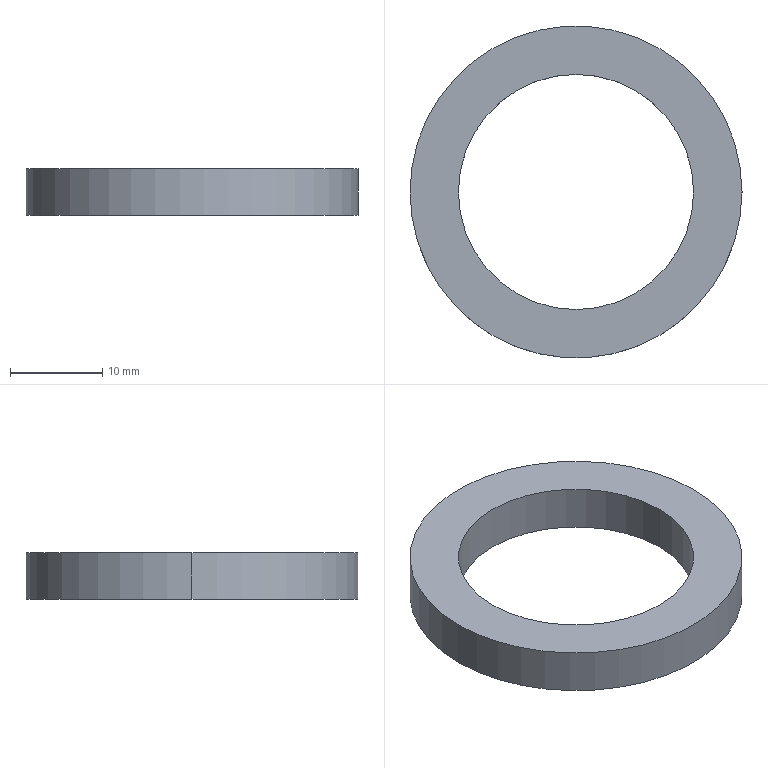Part | SolidWorks | features Extrusion 1 | 1 solid | 6 faces | box 36 x 36 x 5 mm | volume 2536 mm3 | cylinder 4 | plane 2 | commonest cylinder face diameters 25.5 x2 36 x2
STEP:
#1=CARTESIAN_POINT('',(-12.75,0.,5.));
#2=VERTEX_POINT('',#1);
#3=CARTESIAN_POINT('',(12.75,0.,5.));
#4=VERTEX_POINT('',#3);
#5=CARTESIAN_POINT('',(0.,0.,5.));
#6=DIRECTION('',(0.,0.,1.));
#7=DIRECTION('',(1.,0.,0.));
#8=AXIS2_PLACEMENT_3D('',#5,#6,#7);
#9=CIRCLE('',#8,12.75);
#10=EDGE_CURVE('',#2,#4,#9,.T.);
#11=ORIENTED_EDGE('',*,*,#10,.T.);
#12=CARTESIAN_POINT('',(12.75,0.,0.));
#13=VERTEX_POINT('',#12);
#14=CARTESIAN_POINT('',(12.75,0.,5.));
#15=DIRECTION('',(0.,0.,-1.));
#16=VECTOR('',#15,1000.);
#17=LINE('',#14,#16);
#18=EDGE_CURVE('',#4,#13,#17,.T.);
#19=ORIENTED_EDGE('',*,*,#18,.T.);
#20=CARTESIAN_POINT('',(-12.75,0.,0.));
#21=VERTEX_POINT('',#20);
#22=CARTESIAN_POINT('',(0.,0.,0.));
#23=DIRECTION('',(0.,0.,1.));
#24=DIRECTION('',(1.,0.,0.));
#25=AXIS2_PLACEMENT_3D('',#22,#23,#24);
#26=CIRCLE('',#25,12.75);
#27=EDGE_CURVE('',#21,#13,#26,.T.);
#28=ORIENTED_EDGE('',*,*,#27,.F.);
#29=CARTESIAN_POINT('',(-12.75,0.,5.));
#30=DIRECTION('',(0.,0.,-1.));
#31=VECTOR('',#30,1000.);
#32=LINE('',#29,#31);
#33=EDGE_CURVE('',#2,#21,#32,.T.);
#34=ORIENTED_EDGE('',*,*,#33,.F.);
#35=EDGE_LOOP('',(#11,#19,#28,#34));
#36=FACE_OUTER_BOUND('',#35,.T.);
#37=CARTESIAN_POINT('',(0.,0.,5.));
#38=DIRECTION('',(0.,0.,-1.));
#39=DIRECTION('',(-1.,0.,0.));
#40=AXIS2_PLACEMENT_3D('',#37,#38,#39);
#41=CYLINDRICAL_SURFACE('',#40,12.75);
#42=ADVANCED_FACE('',(#36),#41,.F.);
#43=CARTESIAN_POINT('',(18.,0.,5.));
#44=VERTEX_POINT('',#43);
#45=CARTESIAN_POINT('',(-18.,0.,5.));
#46=VERTEX_POINT('',#45);
#47=CARTESIAN_POINT('',(0.,0.,5.));
#48=DIRECTION('',(0.,0.,1.));
#49=DIRECTION('',(1.,0.,0.));
#50=AXIS2_PLACEMENT_3D('',#47,#48,#49);
#51=CIRCLE('',#50,18.);
#52=EDGE_CURVE('',#44,#46,#51,.T.);
#53=ORIENTED_EDGE('',*,*,#52,.F.);
#54=CARTESIAN_POINT('',(18.,0.,0.));
#55=VERTEX_POINT('',#54);
#56=CARTESIAN_POINT('',(18.,0.,5.));
#57=DIRECTION('',(0.,0.,-1.));
#58=VECTOR('',#57,1000.);
#59=LINE('',#56,#58);
#60=EDGE_CURVE('',#44,#55,#59,.T.);
#61=ORIENTED_EDGE('',*,*,#60,.T.);
#62=CARTESIAN_POINT('',(-18.,0.,0.));
#63=VERTEX_POINT('',#62);
#64=CARTESIAN_POINT('',(0.,0.,0.));
#65=DIRECTION('',(0.,0.,1.));
#66=DIRECTION('',(1.,0.,0.));
#67=AXIS2_PLACEMENT_3D('',#64,#65,#66);
#68=CIRCLE('',#67,18.);
#69=EDGE_CURVE('',#55,#63,#68,.T.);
#70=ORIENTED_EDGE('',*,*,#69,.T.);
#71=CARTESIAN_POINT('',(-18.,0.,5.));
#72=DIRECTION('',(0.,0.,-1.));
#73=VECTOR('',#72,1000.);
#74=LINE('',#71,#73);
#75=EDGE_CURVE('',#46,#63,#74,.T.);
#76=ORIENTED_EDGE('',*,*,#75,.F.);
#77=EDGE_LOOP('',(#53,#61,#70,#76));
#78=FACE_OUTER_BOUND('',#77,.T.);
#79=CARTESIAN_POINT('',(0.,0.,5.));
#80=DIRECTION('',(0.,0.,-1.));
#81=DIRECTION('',(-1.,0.,0.));
#82=AXIS2_PLACEMENT_3D('',#79,#80,#81);
#83=CYLINDRICAL_SURFACE('',#82,18.);
#84=ADVANCED_FACE('',(#78),#83,.T.);
#85=CARTESIAN_POINT('',(0.,0.,5.));
#86=DIRECTION('',(0.,0.,1.));
#87=DIRECTION('',(1.,0.,0.));
#88=AXIS2_PLACEMENT_3D('',#85,#86,#87);
#89=CIRCLE('',#88,18.);
#90=EDGE_CURVE('',#46,#44,#89,.T.);
#91=ORIENTED_EDGE('',*,*,#90,.T.);
#92=ORIENTED_EDGE('',*,*,#52,.T.);
#93=EDGE_LOOP('',(#91,#92));
#94=FACE_OUTER_BOUND('',#93,.T.);
#95=ORIENTED_EDGE('',*,*,#10,.F.);
#96=CARTESIAN_POINT('',(0.,0.,5.));
#97=DIRECTION('',(0.,0.,1.));
#98=DIRECTION('',(1.,0.,0.));
#99=AXIS2_PLACEMENT_3D('',#96,#97,#98);
#100=CIRCLE('',#99,12.75);
#101=EDGE_CURVE('',#4,#2,#100,.T.);
#102=ORIENTED_EDGE('',*,*,#101,.F.);
#103=EDGE_LOOP('',(#95,#102));
#104=FACE_BOUND('',#103,.T.);
#105=CARTESIAN_POINT('',(0.,0.,5.));
#106=DIRECTION('',(0.,0.,1.));
#107=DIRECTION('',(1.,0.,0.));
#108=AXIS2_PLACEMENT_3D('',#105,#106,#107);
#109=PLANE('',#108);
#110=ADVANCED_FACE('',(#94,#104),#109,.T.);
#111=CARTESIAN_POINT('',(0.,0.,0.));
#112=DIRECTION('',(0.,0.,1.));
#113=DIRECTION('',(1.,0.,0.));
#114=AXIS2_PLACEMENT_3D('',#111,#112,#113);
#115=CIRCLE('',#114,18.);
#116=EDGE_CURVE('',#63,#55,#115,.T.);
#117=ORIENTED_EDGE('',*,*,#116,.F.);
#118=ORIENTED_EDGE('',*,*,#69,.F.);
#119=EDGE_LOOP('',(#117,#118));
#120=FACE_OUTER_BOUND('',#119,.T.);
#121=ORIENTED_EDGE('',*,*,#27,.T.);
#122=CARTESIAN_POINT('',(0.,0.,0.));
#123=DIRECTION('',(0.,0.,1.));
#124=DIRECTION('',(1.,0.,0.));
#125=AXIS2_PLACEMENT_3D('',#122,#123,#124);
#126=CIRCLE('',#125,12.75);
#127=EDGE_CURVE('',#13,#21,#126,.T.);
#128=ORIENTED_EDGE('',*,*,#127,.T.);
#129=EDGE_LOOP('',(#121,#128));
#130=FACE_BOUND('',#129,.T.);
#131=CARTESIAN_POINT('',(0.,0.,0.));
#132=DIRECTION('',(0.,0.,1.));
#133=DIRECTION('',(1.,0.,0.));
#134=AXIS2_PLACEMENT_3D('',#131,#132,#133);
#135=PLANE('',#134);
#136=ADVANCED_FACE('',(#120,#130),#135,.F.);
#137=ORIENTED_EDGE('',*,*,#60,.F.);
#138=ORIENTED_EDGE('',*,*,#90,.F.);
#139=ORIENTED_EDGE('',*,*,#75,.T.);
#140=ORIENTED_EDGE('',*,*,#116,.T.);
#141=EDGE_LOOP('',(#137,#138,#139,#140));
#142=FACE_OUTER_BOUND('',#141,.T.);
#143=CARTESIAN_POINT('',(0.,0.,5.));
#144=DIRECTION('',(0.,0.,-1.));
#145=DIRECTION('',(-1.,0.,0.));
#146=AXIS2_PLACEMENT_3D('',#143,#144,#145);
#147=CYLINDRICAL_SURFACE('',#146,18.);
#148=ADVANCED_FACE('',(#142),#147,.T.);
#149=ORIENTED_EDGE('',*,*,#18,.F.);
#150=ORIENTED_EDGE('',*,*,#101,.T.);
#151=ORIENTED_EDGE('',*,*,#33,.T.);
#152=ORIENTED_EDGE('',*,*,#127,.F.);
#153=EDGE_LOOP('',(#149,#150,#151,#152));
#154=FACE_OUTER_BOUND('',#153,.T.);
#155=CARTESIAN_POINT('',(0.,0.,5.));
#156=DIRECTION('',(0.,0.,-1.));
#157=DIRECTION('',(-1.,0.,0.));
#158=AXIS2_PLACEMENT_3D('',#155,#156,#157);
#159=CYLINDRICAL_SURFACE('',#158,12.75);
#160=ADVANCED_FACE('',(#154),#159,.F.);
#161=CLOSED_SHELL('',(#42,#84,#110,#136,#148,#160));
#162=MANIFOLD_SOLID_BREP('',#161);
#163=CARTESIAN_POINT('',(0.,0.,0.));
#164=DIRECTION('',(0.,0.,1.));
#165=DIRECTION('',(1.,0.,0.));
#166=AXIS2_PLACEMENT_3D('',#163,#164,#165);
#167=(LENGTH_UNIT()NAMED_UNIT(*)SI_UNIT(.MILLI.,.METRE.));
#168=UNCERTAINTY_MEASURE_WITH_UNIT(LENGTH_MEASURE(0.00001),#167,'','');
#169=(NAMED_UNIT(*)PLANE_ANGLE_UNIT()SI_UNIT($,.RADIAN.));
#170=(NAMED_UNIT(*)SI_UNIT($,.STERADIAN.)SOLID_ANGLE_UNIT());
#171=(GEOMETRIC_REPRESENTATION_CONTEXT(3)GLOBAL_UNCERTAINTY_ASSIGNED_CONTEXT((#168))GLOBAL_UNIT_ASSIGNED_CONTEXT((#167,#169,#170))REPRESENTATION_CONTEXT('',''));
#172=ADVANCED_BREP_SHAPE_REPRESENTATION('',(#162,#166),#171);